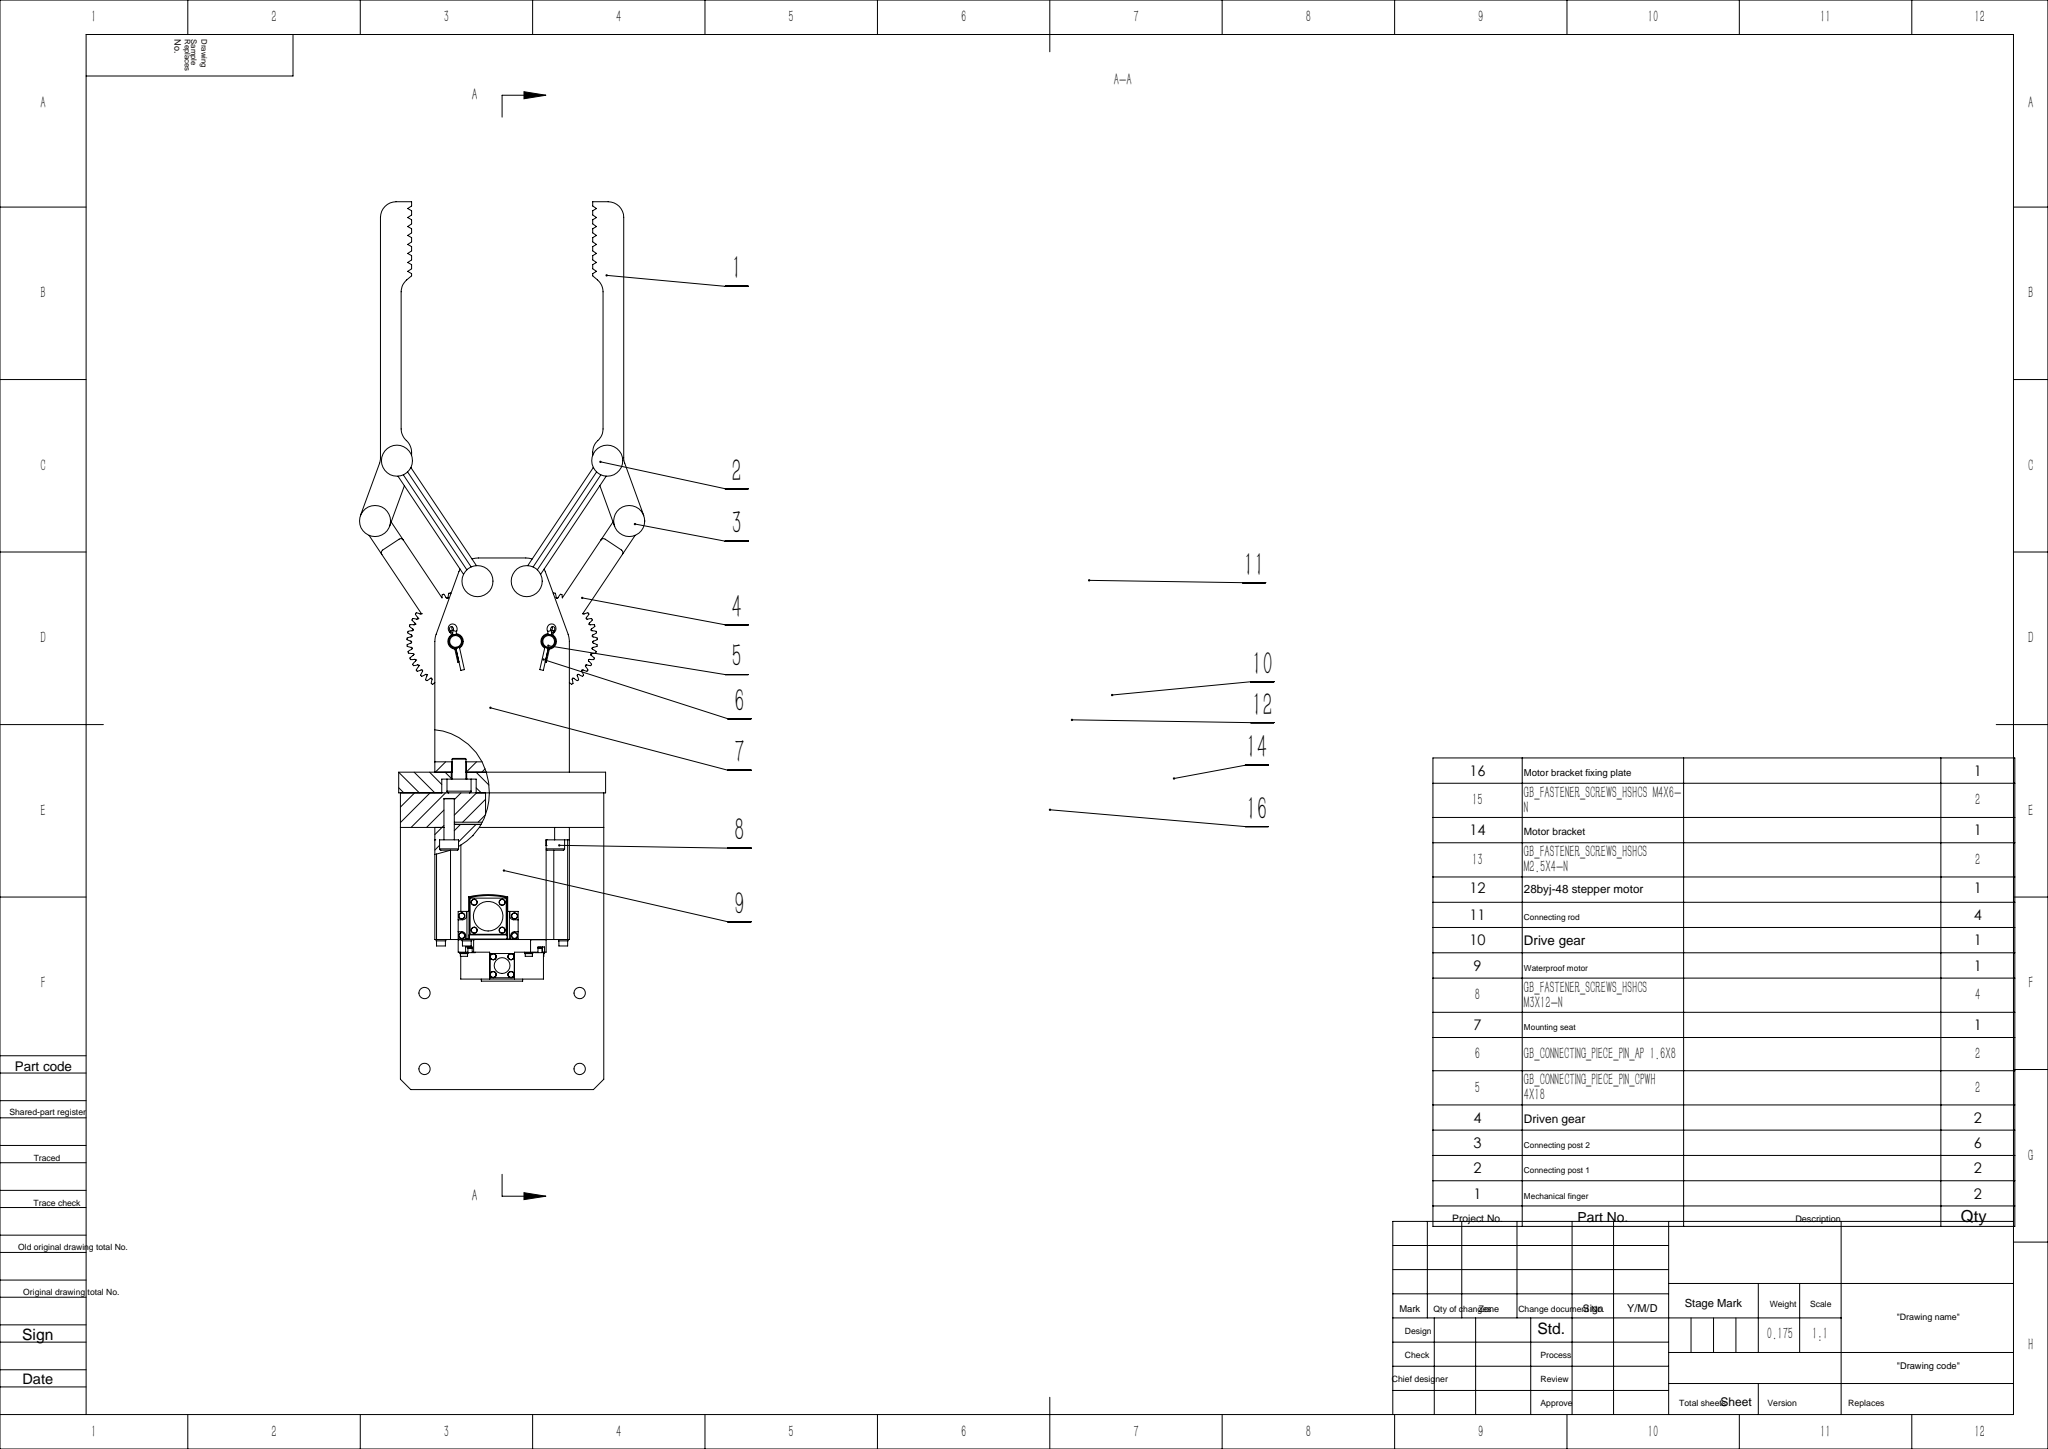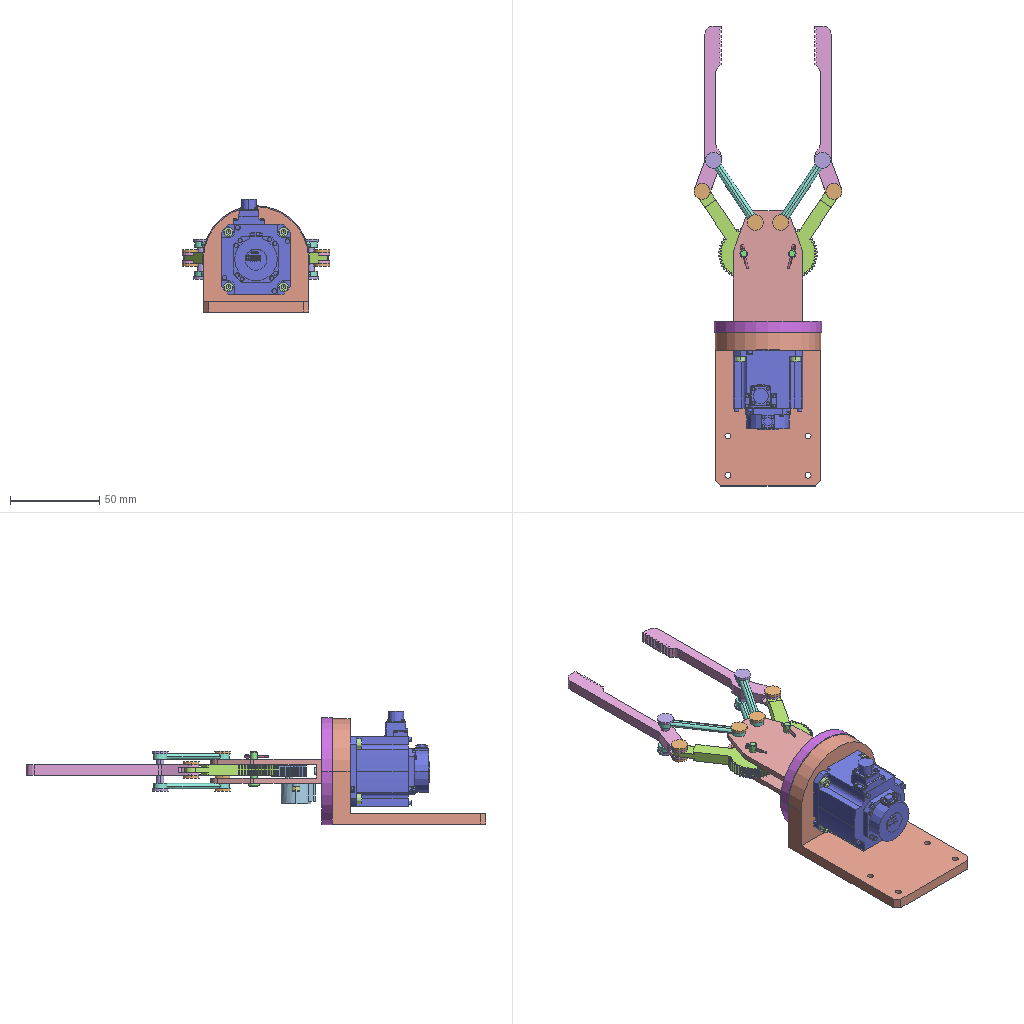Assembly | SolidWorks | 15 different items | 26 placed | box 83 x 257 x 64 mm
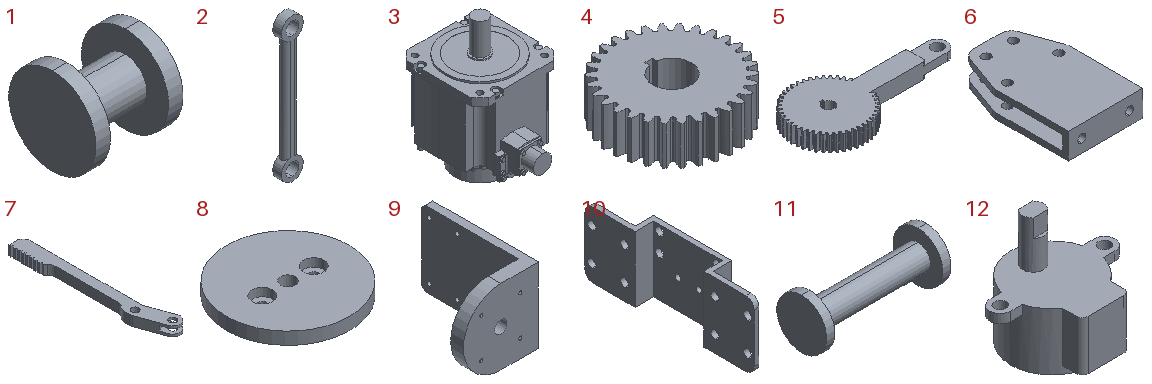Parts list (item | name | quantity | size | volume | features):
1 | - | x6 | 9 x 9 x 9 mm | 286.278 mm3 | features Revolution 1, Scale 1
2 | - | x4 | 7.5 x 3 x 49.5 mm | 573.12 mm3 | features BaseBody 1, HoleWzd 1, Scale 1
3 | - | x1 | 39 x 53.247 x 61.05 mm | 51590 mm3 | features ICE 2, BaseBody 1, Scale 1
4 | - | x1 | 19.181 x 19.198 x 6 mm | 1338 mm3 | features BaseBody 1, Scale 1
5 | - | x2 | 59.85 x 28.19 x 6 mm | 4440 mm3 | features Extrusion 1, Fillet 1, ICE 1, Scale 1
6 | - | x1 | 39 x 62.088 x 13.5 mm | 13319 mm3 | features HoleWzd 5, ICE 5, Fillet 2, Extrusion 1, Scale 1
7 | - | x2 | 15.09 x 97.026 x 6 mm | 3984 mm3 | features HoleWzd 3, ICE 3, Fillet 2, Extrusion 1, Scale 1
8 | - | x1 | 60 x 60 x 6 mm | 16028 mm3 | features Extrusion 1, HoleWzd 1, ICE 1
9 | - | x1 | 59 x 86 x 59 mm | 55181 mm3 | features HoleWzd 2, ICE 2, Chamfer 1, Extrusion 1
10 | - | x1 | 14.25 x 103.05 x 40 mm | 14217 mm3 | features HoleWzd 2, ExtruThin 1, Fillet 1
11 | - | x2 | 22.5 x 9 x 9 mm | 500.986 mm3 | features Revolution 1, Scale 1
12 | - | x1 | 25.2 x 19.2 x 21 mm | 2989 mm3 | features ICE 4, Extrusion 1, Scale 1
13 | clevis pins with head gb | x1 | - | - | -
14 | hexagon socket head cap screws gb | x1 | - | - | -
15 | split pins | x1 | - | - | -
Mates (type | each side: item.copy, entity, surface, feature):
Concentric | 6.1 face cylinder Ø15.0 (15) Diameter Hole2 | 4.1 face cylinder Input1
Width | 4.1 face plane Input1 | 4.1 face plane Input1 | 6.1 face plane Boss-Extrude3 | 6.1 face plane Boss-Extrude1
Concentric | 6.1 face cylinder Ø15.0 (15) Diameter Hole2 | 5.1 face cylinder Boss-Extrude1
Coincident | 6.1 face plane Boss-Extrude3 | 5.1 face plane Boss-Extrude1
Coincident | 5.1 face cylinder Boss-Extrude1 | 7.1 edge
Coincident | 5.1 face plane Cut-Extrude1 | 7.1 face plane Cut-Extrude1
Coincident | 6.1 face plane Boss-Extrude3 | 2.1 face plane Input3
Concentric | 7.1 face cylinder Ø15.0 (15) Diameter Hole2 | 2.1 face cylinder Ø15.0 (15) Diameter Hole1
Concentric | 6.1 face cylinder Ø15.0 (15) Diameter Hole1 | 2.1 face cylinder Ø15.0 (15) Diameter Hole1
Concentric | 7.1 face cylinder Ø15.0 (15) Diameter Hole3 | 1.1 face cylinder Revolve1
Coincident | 7.1 face plane Boss-Extrude1 | 1.1 face plane Revolve1
Concentric | 7.1 face cylinder Ø15.0 (15) Diameter Hole2 | 11.1 face cylinder Revolve1
Coincident | 2.1 face plane Input3 | 11.1 face plane Revolve1
Coincident | 6.1 face plane Boss-Extrude1 | 2.2 face plane Input3
Concentric | 6.1 face cylinder Ø15.0 (15) Diameter Hole2 | 2.2 face cylinder Ø15.0 (15) Diameter Hole1
Concentric | 11.1 face cylinder Revolve1 | 2.2 face cylinder Ø15.0 (15) Diameter Hole1
Concentric | 6.1 face cylinder Ø15.0 (15) Diameter Hole1 | 1.2 face cylinder Revolve1
Coincident | 6.1 face plane Boss-Extrude3 | 1.2 face plane Revolve1
Coincident | 6.1 face plane Boss-Extrude1 | 1.3 face plane Revolve1
Concentric | 6.1 face cylinder Ø15.0 (15) Diameter Hole2 | 1.3 face cylinder Revolve1
Concentric | 6.1 face cylinder Ø15.0 (15) Diameter Hole2 | 12.1 face cylinder Boss-Extrude3
Coincident | 6.1 face plane Boss-Extrude1 | 12.1 face plane Boss-Extrude1
Concentric | 6.1 face cylinder M5 Tapped Hole1 | 8.1 face cylinder CBORE for M4 Hex Head Bolt1 | 2 times
Coincident | 6.1 face plane Boss-Extrude1 | 8.1 face plane Boss-Extrude1
Coincident | 8.1 face plane Boss-Extrude1 | 9.1 face plane Boss-Extrude1
Concentric | 9.1 face cylinder Cut-Extrude2 | 3.1 face cylinder Input1
Coincident | 9.1 face plane Boss-Extrude1 | 3.1 face plane Input1
Parallel | 9.1 face plane Boss-Extrude1 | 3.1 face plane Input1